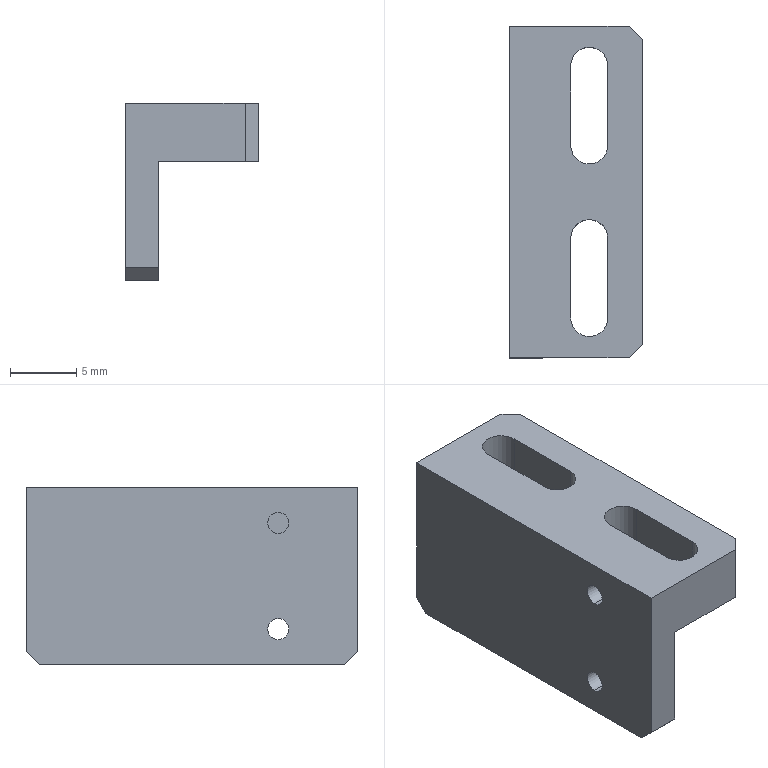Part | SolidWorks | features Chamfer 1, Cut 1, Extrusion 1, HoleWzd 1, ICE 1 | 1 solid | 24 faces | box 10 x 25 x 13.4 mm | volume 1439 mm3 | plane 16 | cylinder 8 | commonest cylinder face diameters 1.6 x4 2.8 x4
STEP:
#1=CARTESIAN_POINT('',(2.5,6.,-9.9));
#2=VERTEX_POINT('',#1);
#3=CARTESIAN_POINT('',(2.5,6.,-11.5));
#4=VERTEX_POINT('',#3);
#5=CARTESIAN_POINT('',(2.5,6.,-10.7));
#6=DIRECTION('',(1.,0.,0.));
#7=DIRECTION('',(0.,0.,1.));
#8=AXIS2_PLACEMENT_3D('',#5,#6,#7);
#9=CIRCLE('',#8,0.8);
#10=EDGE_CURVE('',#2,#4,#9,.T.);
#11=ORIENTED_EDGE('',*,*,#10,.T.);
#12=CARTESIAN_POINT('',(0.,6.,-11.5));
#13=VERTEX_POINT('',#12);
#14=CARTESIAN_POINT('',(0.,6.,-11.5));
#15=DIRECTION('',(-1.,0.,0.));
#16=VECTOR('',#15,1000.);
#17=LINE('',#14,#16);
#18=EDGE_CURVE('',#4,#13,#17,.T.);
#19=ORIENTED_EDGE('',*,*,#18,.T.);
#20=CARTESIAN_POINT('',(0.,6.,-9.9));
#21=VERTEX_POINT('',#20);
#22=CARTESIAN_POINT('',(0.,6.,-10.7));
#23=DIRECTION('',(-1.,0.,0.));
#24=DIRECTION('',(0.,0.,1.));
#25=AXIS2_PLACEMENT_3D('',#22,#23,#24);
#26=CIRCLE('',#25,0.8);
#27=EDGE_CURVE('',#13,#21,#26,.T.);
#28=ORIENTED_EDGE('',*,*,#27,.T.);
#29=CARTESIAN_POINT('',(0.,6.,-9.9));
#30=DIRECTION('',(-1.,0.,0.));
#31=VECTOR('',#30,1000.);
#32=LINE('',#29,#31);
#33=EDGE_CURVE('',#2,#21,#32,.T.);
#34=ORIENTED_EDGE('',*,*,#33,.F.);
#35=EDGE_LOOP('',(#11,#19,#28,#34));
#36=FACE_OUTER_BOUND('',#35,.T.);
#37=CARTESIAN_POINT('',(0.,6.,-10.7));
#38=DIRECTION('',(-1.,0.,0.));
#39=DIRECTION('',(0.,0.,1.));
#40=AXIS2_PLACEMENT_3D('',#37,#38,#39);
#41=CYLINDRICAL_SURFACE('',#40,0.8);
#42=ADVANCED_FACE('',(#36),#41,.F.);
#43=CARTESIAN_POINT('',(4.6,6.,-3.5));
#44=VERTEX_POINT('',#43);
#45=CARTESIAN_POINT('',(4.6,6.,-1.9));
#46=VERTEX_POINT('',#45);
#47=CARTESIAN_POINT('',(4.6,6.,-2.7));
#48=DIRECTION('',(-1.,0.,0.));
#49=DIRECTION('',(0.,0.,1.));
#50=AXIS2_PLACEMENT_3D('',#47,#48,#49);
#51=CIRCLE('',#50,0.8);
#52=EDGE_CURVE('',#44,#46,#51,.T.);
#53=ORIENTED_EDGE('',*,*,#52,.F.);
#54=CARTESIAN_POINT('',(0.,6.,-3.5));
#55=VERTEX_POINT('',#54);
#56=CARTESIAN_POINT('',(0.,6.,-3.5));
#57=DIRECTION('',(-1.,0.,0.));
#58=VECTOR('',#57,1000.);
#59=LINE('',#56,#58);
#60=EDGE_CURVE('',#44,#55,#59,.T.);
#61=ORIENTED_EDGE('',*,*,#60,.T.);
#62=CARTESIAN_POINT('',(0.,6.,-1.9));
#63=VERTEX_POINT('',#62);
#64=CARTESIAN_POINT('',(0.,6.,-2.7));
#65=DIRECTION('',(-1.,0.,0.));
#66=DIRECTION('',(0.,0.,1.));
#67=AXIS2_PLACEMENT_3D('',#64,#65,#66);
#68=CIRCLE('',#67,0.8);
#69=EDGE_CURVE('',#55,#63,#68,.T.);
#70=ORIENTED_EDGE('',*,*,#69,.T.);
#71=CARTESIAN_POINT('',(0.,6.,-1.9));
#72=DIRECTION('',(-1.,0.,0.));
#73=VECTOR('',#72,1000.);
#74=LINE('',#71,#73);
#75=EDGE_CURVE('',#46,#63,#74,.T.);
#76=ORIENTED_EDGE('',*,*,#75,.F.);
#77=EDGE_LOOP('',(#53,#61,#70,#76));
#78=FACE_OUTER_BOUND('',#77,.T.);
#79=CARTESIAN_POINT('',(0.,6.,-2.7));
#80=DIRECTION('',(-1.,0.,0.));
#81=DIRECTION('',(0.,0.,1.));
#82=AXIS2_PLACEMENT_3D('',#79,#80,#81);
#83=CYLINDRICAL_SURFACE('',#82,0.8);
#84=ADVANCED_FACE('',(#78),#83,.F.);
#85=CARTESIAN_POINT('',(0.,6.,-10.7));
#86=DIRECTION('',(-1.,0.,0.));
#87=DIRECTION('',(0.,0.,1.));
#88=AXIS2_PLACEMENT_3D('',#85,#86,#87);
#89=CIRCLE('',#88,0.8);
#90=EDGE_CURVE('',#21,#13,#89,.T.);
#91=ORIENTED_EDGE('',*,*,#90,.F.);
#92=ORIENTED_EDGE('',*,*,#27,.F.);
#93=EDGE_LOOP('',(#91,#92));
#94=FACE_BOUND('',#93,.T.);
#95=CARTESIAN_POINT('',(0.,6.,-2.7));
#96=DIRECTION('',(-1.,0.,0.));
#97=DIRECTION('',(0.,0.,1.));
#98=AXIS2_PLACEMENT_3D('',#95,#96,#97);
#99=CIRCLE('',#98,0.8);
#100=EDGE_CURVE('',#63,#55,#99,.T.);
#101=ORIENTED_EDGE('',*,*,#100,.F.);
#102=ORIENTED_EDGE('',*,*,#69,.F.);
#103=EDGE_LOOP('',(#101,#102));
#104=FACE_BOUND('',#103,.T.);
#105=CARTESIAN_POINT('',(0.,24.,-13.4));
#106=VERTEX_POINT('',#105);
#107=CARTESIAN_POINT('',(0.,1.,-13.4));
#108=VERTEX_POINT('',#107);
#109=CARTESIAN_POINT('',(0.,25.,-13.4));
#110=DIRECTION('',(0.,-1.,0.));
#111=VECTOR('',#110,1000.);
#112=LINE('',#109,#111);
#113=EDGE_CURVE('',#106,#108,#112,.T.);
#114=ORIENTED_EDGE('',*,*,#113,.T.);
#115=CARTESIAN_POINT('',(0.,0.,-12.4));
#116=VERTEX_POINT('',#115);
#117=CARTESIAN_POINT('',(0.,1.,-13.4));
#118=DIRECTION('',(0.,-0.7071,0.7071));
#119=VECTOR('',#118,1000.);
#120=LINE('',#117,#119);
#121=EDGE_CURVE('',#108,#116,#120,.T.);
#122=ORIENTED_EDGE('',*,*,#121,.T.);
#123=CARTESIAN_POINT('',(0.,0.,0.));
#124=VERTEX_POINT('',#123);
#125=CARTESIAN_POINT('',(0.,0.,0.));
#126=DIRECTION('',(0.,0.,1.));
#127=VECTOR('',#126,1000.);
#128=LINE('',#125,#127);
#129=EDGE_CURVE('',#116,#124,#128,.T.);
#130=ORIENTED_EDGE('',*,*,#129,.T.);
#131=CARTESIAN_POINT('',(0.,25.,0.));
#132=VERTEX_POINT('',#131);
#133=CARTESIAN_POINT('',(0.,25.,0.));
#134=DIRECTION('',(0.,-1.,0.));
#135=VECTOR('',#134,1000.);
#136=LINE('',#133,#135);
#137=EDGE_CURVE('',#132,#124,#136,.T.);
#138=ORIENTED_EDGE('',*,*,#137,.F.);
#139=CARTESIAN_POINT('',(0.,25.,-12.4));
#140=VERTEX_POINT('',#139);
#141=CARTESIAN_POINT('',(0.,25.,0.));
#142=DIRECTION('',(0.,0.,1.));
#143=VECTOR('',#142,1000.);
#144=LINE('',#141,#143);
#145=EDGE_CURVE('',#140,#132,#144,.T.);
#146=ORIENTED_EDGE('',*,*,#145,.F.);
#147=CARTESIAN_POINT('',(0.,25.,-12.4));
#148=DIRECTION('',(0.,-0.7071,-0.7071));
#149=VECTOR('',#148,1000.);
#150=LINE('',#147,#149);
#151=EDGE_CURVE('',#140,#106,#150,.T.);
#152=ORIENTED_EDGE('',*,*,#151,.T.);
#153=EDGE_LOOP('',(#114,#122,#130,#138,#146,#152));
#154=FACE_OUTER_BOUND('',#153,.T.);
#155=CARTESIAN_POINT('',(0.,25.,0.));
#156=DIRECTION('',(1.,0.,0.));
#157=DIRECTION('',(0.,0.,-1.));
#158=AXIS2_PLACEMENT_3D('',#155,#156,#157);
#159=PLANE('',#158);
#160=ADVANCED_FACE('',(#94,#104,#154),#159,.F.);
#161=CARTESIAN_POINT('',(7.4,3.,0.));
#162=VERTEX_POINT('',#161);
#163=CARTESIAN_POINT('',(7.4,9.,0.));
#164=VERTEX_POINT('',#163);
#165=CARTESIAN_POINT('',(7.4,3.,0.));
#166=DIRECTION('',(0.,1.,0.));
#167=VECTOR('',#166,1000.);
#168=LINE('',#165,#167);
#169=EDGE_CURVE('',#162,#164,#168,.T.);
#170=ORIENTED_EDGE('',*,*,#169,.F.);
#171=CARTESIAN_POINT('',(4.6,3.,0.));
#172=VERTEX_POINT('',#171);
#173=CARTESIAN_POINT('',(6.,3.,0.));
#174=DIRECTION('',(0.,0.,1.));
#175=DIRECTION('',(-1.,0.,0.));
#176=AXIS2_PLACEMENT_3D('',#173,#174,#175);
#177=CIRCLE('',#176,1.4);
#178=EDGE_CURVE('',#172,#162,#177,.T.);
#179=ORIENTED_EDGE('',*,*,#178,.F.);
#180=CARTESIAN_POINT('',(4.6,9.,0.));
#181=VERTEX_POINT('',#180);
#182=CARTESIAN_POINT('',(4.6,3.,0.));
#183=DIRECTION('',(0.,-1.,0.));
#184=VECTOR('',#183,1000.);
#185=LINE('',#182,#184);
#186=EDGE_CURVE('',#181,#172,#185,.T.);
#187=ORIENTED_EDGE('',*,*,#186,.F.);
#188=CARTESIAN_POINT('',(6.,9.,0.));
#189=DIRECTION('',(0.,0.,1.));
#190=DIRECTION('',(-1.,0.,0.));
#191=AXIS2_PLACEMENT_3D('',#188,#189,#190);
#192=CIRCLE('',#191,1.4);
#193=EDGE_CURVE('',#164,#181,#192,.T.);
#194=ORIENTED_EDGE('',*,*,#193,.F.);
#195=EDGE_LOOP('',(#170,#179,#187,#194));
#196=FACE_BOUND('',#195,.T.);
#197=CARTESIAN_POINT('',(4.6,22.,0.));
#198=VERTEX_POINT('',#197);
#199=CARTESIAN_POINT('',(4.6,16.,0.));
#200=VERTEX_POINT('',#199);
#201=CARTESIAN_POINT('',(4.6,22.,0.));
#202=DIRECTION('',(0.,-1.,0.));
#203=VECTOR('',#202,1000.);
#204=LINE('',#201,#203);
#205=EDGE_CURVE('',#198,#200,#204,.T.);
#206=ORIENTED_EDGE('',*,*,#205,.F.);
#207=CARTESIAN_POINT('',(7.4,22.,0.));
#208=VERTEX_POINT('',#207);
#209=CARTESIAN_POINT('',(6.,22.,0.));
#210=DIRECTION('',(0.,0.,1.));
#211=DIRECTION('',(1.,0.,0.));
#212=AXIS2_PLACEMENT_3D('',#209,#210,#211);
#213=CIRCLE('',#212,1.4);
#214=EDGE_CURVE('',#208,#198,#213,.T.);
#215=ORIENTED_EDGE('',*,*,#214,.F.);
#216=CARTESIAN_POINT('',(7.4,16.,0.));
#217=VERTEX_POINT('',#216);
#218=CARTESIAN_POINT('',(7.4,22.,0.));
#219=DIRECTION('',(0.,1.,0.));
#220=VECTOR('',#219,1000.);
#221=LINE('',#218,#220);
#222=EDGE_CURVE('',#217,#208,#221,.T.);
#223=ORIENTED_EDGE('',*,*,#222,.F.);
#224=CARTESIAN_POINT('',(6.,16.,0.));
#225=DIRECTION('',(0.,0.,1.));
#226=DIRECTION('',(1.,0.,0.));
#227=AXIS2_PLACEMENT_3D('',#224,#225,#226);
#228=CIRCLE('',#227,1.4);
#229=EDGE_CURVE('',#200,#217,#228,.T.);
#230=ORIENTED_EDGE('',*,*,#229,.F.);
#231=EDGE_LOOP('',(#206,#215,#223,#230));
#232=FACE_BOUND('',#231,.T.);
#233=CARTESIAN_POINT('',(9.,0.,0.));
#234=VERTEX_POINT('',#233);
#235=CARTESIAN_POINT('',(0.,0.,0.));
#236=DIRECTION('',(1.,0.,0.));
#237=VECTOR('',#236,1000.);
#238=LINE('',#235,#237);
#239=EDGE_CURVE('',#124,#234,#238,.T.);
#240=ORIENTED_EDGE('',*,*,#239,.T.);
#241=CARTESIAN_POINT('',(10.,1.,0.));
#242=VERTEX_POINT('',#241);
#243=CARTESIAN_POINT('',(10.,1.,0.));
#244=DIRECTION('',(0.7071,0.7071,0.));
#245=VECTOR('',#244,1000.);
#246=LINE('',#243,#245);
#247=EDGE_CURVE('',#234,#242,#246,.T.);
#248=ORIENTED_EDGE('',*,*,#247,.T.);
#249=CARTESIAN_POINT('',(10.,24.,0.));
#250=VERTEX_POINT('',#249);
#251=CARTESIAN_POINT('',(10.,25.,0.));
#252=DIRECTION('',(0.,-1.,0.));
#253=VECTOR('',#252,1000.);
#254=LINE('',#251,#253);
#255=EDGE_CURVE('',#250,#242,#254,.T.);
#256=ORIENTED_EDGE('',*,*,#255,.F.);
#257=CARTESIAN_POINT('',(9.,25.,0.));
#258=VERTEX_POINT('',#257);
#259=CARTESIAN_POINT('',(9.,25.,0.));
#260=DIRECTION('',(-0.7071,0.7071,0.));
#261=VECTOR('',#260,1000.);
#262=LINE('',#259,#261);
#263=EDGE_CURVE('',#250,#258,#262,.T.);
#264=ORIENTED_EDGE('',*,*,#263,.T.);
#265=CARTESIAN_POINT('',(0.,25.,0.));
#266=DIRECTION('',(1.,0.,0.));
#267=VECTOR('',#266,1000.);
#268=LINE('',#265,#267);
#269=EDGE_CURVE('',#132,#258,#268,.T.);
#270=ORIENTED_EDGE('',*,*,#269,.F.);
#271=ORIENTED_EDGE('',*,*,#137,.T.);
#272=EDGE_LOOP('',(#240,#248,#256,#264,#270,#271));
#273=FACE_OUTER_BOUND('',#272,.T.);
#274=CARTESIAN_POINT('',(0.,25.,0.));
#275=DIRECTION('',(0.,0.,-1.));
#276=DIRECTION('',(-1.,0.,0.));
#277=AXIS2_PLACEMENT_3D('',#274,#275,#276);
#278=PLANE('',#277);
#279=ADVANCED_FACE('',(#196,#232,#273),#278,.F.);
#280=ORIENTED_EDGE('',*,*,#255,.T.);
#281=CARTESIAN_POINT('',(10.,1.,-4.4));
#282=VERTEX_POINT('',#281);
#283=CARTESIAN_POINT('',(10.,1.,-4.4));
#284=DIRECTION('',(0.,0.,-1.));
#285=VECTOR('',#284,1000.);
#286=LINE('',#283,#285);
#287=EDGE_CURVE('',#242,#282,#286,.T.);
#288=ORIENTED_EDGE('',*,*,#287,.T.);
#289=CARTESIAN_POINT('',(10.,24.,-4.4));
#290=VERTEX_POINT('',#289);
#291=CARTESIAN_POINT('',(10.,25.,-4.4));
#292=DIRECTION('',(0.,1.,0.));
#293=VECTOR('',#292,1000.);
#294=LINE('',#291,#293);
#295=EDGE_CURVE('',#282,#290,#294,.T.);
#296=ORIENTED_EDGE('',*,*,#295,.T.);
#297=CARTESIAN_POINT('',(10.,24.,0.));
#298=DIRECTION('',(0.,0.,1.));
#299=VECTOR('',#298,1000.);
#300=LINE('',#297,#299);
#301=EDGE_CURVE('',#290,#250,#300,.T.);
#302=ORIENTED_EDGE('',*,*,#301,.T.);
#303=EDGE_LOOP('',(#280,#288,#296,#302));
#304=FACE_OUTER_BOUND('',#303,.T.);
#305=CARTESIAN_POINT('',(10.,25.,0.));
#306=DIRECTION('',(-1.,0.,0.));
#307=DIRECTION('',(0.,0.,1.));
#308=AXIS2_PLACEMENT_3D('',#305,#306,#307);
#309=PLANE('',#308);
#310=ADVANCED_FACE('',(#304),#309,.F.);
#311=CARTESIAN_POINT('',(2.5,1.,-13.4));
#312=VERTEX_POINT('',#311);
#313=CARTESIAN_POINT('',(2.5,24.,-13.4));
#314=VERTEX_POINT('',#313);
#315=CARTESIAN_POINT('',(2.5,25.,-13.4));
#316=DIRECTION('',(0.,1.,0.));
#317=VECTOR('',#316,1000.);
#318=LINE('',#315,#317);
#319=EDGE_CURVE('',#312,#314,#318,.T.);
#320=ORIENTED_EDGE('',*,*,#319,.F.);
#321=CARTESIAN_POINT('',(0.,1.,-13.4));
#322=DIRECTION('',(-1.,0.,0.));
#323=VECTOR('',#322,1000.);
#324=LINE('',#321,#323);
#325=EDGE_CURVE('',#312,#108,#324,.T.);
#326=ORIENTED_EDGE('',*,*,#325,.T.);
#327=ORIENTED_EDGE('',*,*,#113,.F.);
#328=CARTESIAN_POINT('',(0.,24.,-13.4));
#329=DIRECTION('',(1.,0.,0.));
#330=VECTOR('',#329,1000.);
#331=LINE('',#328,#330);
#332=EDGE_CURVE('',#106,#314,#331,.T.);
#333=ORIENTED_EDGE('',*,*,#332,.T.);
#334=EDGE_LOOP('',(#320,#326,#327,#333));
#335=FACE_OUTER_BOUND('',#334,.T.);
#336=CARTESIAN_POINT('',(0.,25.,-13.4));
#337=DIRECTION('',(0.,0.,1.));
#338=DIRECTION('',(1.,0.,0.));
#339=AXIS2_PLACEMENT_3D('',#336,#337,#338);
#340=PLANE('',#339);
#341=ADVANCED_FACE('',(#335),#340,.F.);
#342=CARTESIAN_POINT('',(2.5,25.,-4.4));
#343=VERTEX_POINT('',#342);
#344=CARTESIAN_POINT('',(2.5,25.,-12.4));
#345=VERTEX_POINT('',#344);
#346=CARTESIAN_POINT('',(2.5,25.,-4.4));
#347=DIRECTION('',(0.,0.,-1.));
#348=VECTOR('',#347,1000.);
#349=LINE('',#346,#348);
#350=EDGE_CURVE('',#343,#345,#349,.T.);
#351=ORIENTED_EDGE('',*,*,#350,.T.);
#352=CARTESIAN_POINT('',(0.,25.,-12.4));
#353=DIRECTION('',(-1.,0.,0.));
#354=VECTOR('',#353,1000.);
#355=LINE('',#352,#354);
#356=EDGE_CURVE('',#345,#140,#355,.T.);
#357=ORIENTED_EDGE('',*,*,#356,.T.);
#358=ORIENTED_EDGE('',*,*,#145,.T.);
#359=ORIENTED_EDGE('',*,*,#269,.T.);
#360=CARTESIAN_POINT('',(9.,25.,-4.4));
#361=VERTEX_POINT('',#360);
#362=CARTESIAN_POINT('',(9.,25.,0.));
#363=DIRECTION('',(0.,0.,-1.));
#364=VECTOR('',#363,1000.);
#365=LINE('',#362,#364);
#366=EDGE_CURVE('',#258,#361,#365,.T.);
#367=ORIENTED_EDGE('',*,*,#366,.T.);
#368=CARTESIAN_POINT('',(2.5,25.,-4.4));
#369=DIRECTION('',(1.,0.,0.));
#370=VECTOR('',#369,1000.);
#371=LINE('',#368,#370);
#372=EDGE_CURVE('',#343,#361,#371,.T.);
#373=ORIENTED_EDGE('',*,*,#372,.F.);
#374=EDGE_LOOP('',(#351,#357,#358,#359,#367,#373));
#375=FACE_OUTER_BOUND('',#374,.T.);
#376=CARTESIAN_POINT('',(0.,25.,0.));
#377=DIRECTION('',(0.,-1.,0.));
#378=DIRECTION('',(0.,0.,-1.));
#379=AXIS2_PLACEMENT_3D('',#376,#377,#378);
#380=PLANE('',#379);
#381=ADVANCED_FACE('',(#375),#380,.F.);
#382=ORIENTED_EDGE('',*,*,#129,.F.);
#383=CARTESIAN_POINT('',(2.5,0.,-12.4));
#384=VERTEX_POINT('',#383);
#385=CARTESIAN_POINT('',(2.5,0.,-12.4));
#386=DIRECTION('',(1.,0.,0.));
#387=VECTOR('',#386,1000.);
#388=LINE('',#385,#387);
#389=EDGE_CURVE('',#116,#384,#388,.T.);
#390=ORIENTED_EDGE('',*,*,#389,.T.);
#391=CARTESIAN_POINT('',(2.5,0.,-4.4));
#392=VERTEX_POINT('',#391);
#393=CARTESIAN_POINT('',(2.5,0.,-4.4));
#394=DIRECTION('',(0.,0.,-1.));
#395=VECTOR('',#394,1000.);
#396=LINE('',#393,#395);
#397=EDGE_CURVE('',#392,#384,#396,.T.);
#398=ORIENTED_EDGE('',*,*,#397,.F.);
#399=CARTESIAN_POINT('',(9.,0.,-4.4));
#400=VERTEX_POINT('',#399);
#401=CARTESIAN_POINT('',(2.5,0.,-4.4));
#402=DIRECTION('',(-1.,0.,0.));
#403=VECTOR('',#402,1000.);
#404=LINE('',#401,#403);
#405=EDGE_CURVE('',#400,#392,#404,.T.);
#406=ORIENTED_EDGE('',*,*,#405,.F.);
#407=CARTESIAN_POINT('',(9.,0.,0.));
#408=DIRECTION('',(0.,0.,1.));
#409=VECTOR('',#408,1000.);
#410=LINE('',#407,#409);
#411=EDGE_CURVE('',#400,#234,#410,.T.);
#412=ORIENTED_EDGE('',*,*,#411,.T.);
#413=ORIENTED_EDGE('',*,*,#239,.F.);
#414=EDGE_LOOP('',(#382,#390,#398,#406,#412,#413));
#415=FACE_OUTER_BOUND('',#414,.T.);
#416=CARTESIAN_POINT('',(0.,0.,0.));
#417=DIRECTION('',(0.,-1.,0.));
#418=DIRECTION('',(0.,0.,-1.));
#419=AXIS2_PLACEMENT_3D('',#416,#417,#418);
#420=PLANE('',#419);
#421=ADVANCED_FACE('',(#415),#420,.T.);
#422=CARTESIAN_POINT('',(4.6,22.,-4.4));
#423=VERTEX_POINT('',#422);
#424=CARTESIAN_POINT('',(4.6,22.,-14.));
#425=DIRECTION('',(0.,0.,1.));
#426=VECTOR('',#425,1000.);
#427=LINE('',#424,#426);
#428=EDGE_CURVE('',#423,#198,#427,.T.);
#429=ORIENTED_EDGE('',*,*,#428,.F.);
#430=CARTESIAN_POINT('',(7.4,22.,-4.4));
#431=VERTEX_POINT('',#430);
#432=CARTESIAN_POINT('',(6.,22.,-4.4));
#433=DIRECTION('',(0.,0.,-1.));
#434=DIRECTION('',(1.,0.,0.));
#435=AXIS2_PLACEMENT_3D('',#432,#433,#434);
#436=CIRCLE('',#435,1.4);
#437=EDGE_CURVE('',#423,#431,#436,.T.);
#438=ORIENTED_EDGE('',*,*,#437,.T.);
#439=CARTESIAN_POINT('',(7.4,22.,-14.));
#440=DIRECTION('',(0.,0.,1.));
#441=VECTOR('',#440,1000.);
#442=LINE('',#439,#441);
#443=EDGE_CURVE('',#431,#208,#442,.T.);
#444=ORIENTED_EDGE('',*,*,#443,.T.);
#445=ORIENTED_EDGE('',*,*,#214,.T.);
#446=EDGE_LOOP('',(#429,#438,#444,#445));
#447=FACE_OUTER_BOUND('',#446,.T.);
#448=CARTESIAN_POINT('',(6.,22.,-14.));
#449=DIRECTION('',(0.,0.,1.));
#450=DIRECTION('',(1.,0.,0.));
#451=AXIS2_PLACEMENT_3D('',#448,#449,#450);
#452=CYLINDRICAL_SURFACE('',#451,1.4);
#453=ADVANCED_FACE('',(#447),#452,.F.);
#454=ORIENTED_EDGE('',*,*,#443,.F.);
#455=CARTESIAN_POINT('',(7.4,16.,-4.4));
#456=VERTEX_POINT('',#455);
#457=CARTESIAN_POINT('',(7.4,22.,-4.4));
#458=DIRECTION('',(0.,-1.,0.));
#459=VECTOR('',#458,1000.);
#460=LINE('',#457,#459);
#461=EDGE_CURVE('',#431,#456,#460,.T.);
#462=ORIENTED_EDGE('',*,*,#461,.T.);
#463=CARTESIAN_POINT('',(7.4,16.,-14.));
#464=DIRECTION('',(0.,0.,1.));
#465=VECTOR('',#464,1000.);
#466=LINE('',#463,#465);
#467=EDGE_CURVE('',#456,#217,#466,.T.);
#468=ORIENTED_EDGE('',*,*,#467,.T.);
#469=ORIENTED_EDGE('',*,*,#222,.T.);
#470=EDGE_LOOP('',(#454,#462,#468,#469));
#471=FACE_OUTER_BOUND('',#470,.T.);
#472=CARTESIAN_POINT('',(7.4,22.,-14.));
#473=DIRECTION('',(1.,0.,0.));
#474=DIRECTION('',(0.,0.,-1.));
#475=AXIS2_PLACEMENT_3D('',#472,#473,#474);
#476=PLANE('',#475);
#477=ADVANCED_FACE('',(#471),#476,.F.);
#478=ORIENTED_EDGE('',*,*,#467,.F.);
#479=CARTESIAN_POINT('',(4.6,16.,-4.4));
#480=VERTEX_POINT('',#479);
#481=CARTESIAN_POINT('',(6.,16.,-4.4));
#482=DIRECTION('',(0.,0.,-1.));
#483=DIRECTION('',(1.,0.,0.));
#484=AXIS2_PLACEMENT_3D('',#481,#482,#483);
#485=CIRCLE('',#484,1.4);
#486=EDGE_CURVE('',#456,#480,#485,.T.);
#487=ORIENTED_EDGE('',*,*,#486,.T.);
#488=CARTESIAN_POINT('',(4.6,16.,-14.));
#489=DIRECTION('',(0.,0.,1.));
#490=VECTOR('',#489,1000.);
#491=LINE('',#488,#490);
#492=EDGE_CURVE('',#480,#200,#491,.T.);
#493=ORIENTED_EDGE('',*,*,#492,.T.);
#494=ORIENTED_EDGE('',*,*,#229,.T.);
#495=EDGE_LOOP('',(#478,#487,#493,#494));
#496=FACE_OUTER_BOUND('',#495,.T.);
#497=CARTESIAN_POINT('',(6.,16.,-14.));
#498=DIRECTION('',(0.,0.,1.));
#499=DIRECTION('',(1.,0.,0.));
#500=AXIS2_PLACEMENT_3D('',#497,#498,#499);
#501=CYLINDRICAL_SURFACE('',#500,1.4);
#502=ADVANCED_FACE('',(#496),#501,.F.);
#503=ORIENTED_EDGE('',*,*,#492,.F.);
#504=CARTESIAN_POINT('',(4.6,22.,-4.4));
#505=DIRECTION('',(0.,1.,0.));
#506=VECTOR('',#505,1000.);
#507=LINE('',#504,#506);
#508=EDGE_CURVE('',#480,#423,#507,.T.);
#509=ORIENTED_EDGE('',*,*,#508,.T.);
#510=ORIENTED_EDGE('',*,*,#428,.T.);
#511=ORIENTED_EDGE('',*,*,#205,.T.);
#512=EDGE_LOOP('',(#503,#509,#510,#511));
#513=FACE_OUTER_BOUND('',#512,.T.);
#514=CARTESIAN_POINT('',(4.6,22.,-14.));
#515=DIRECTION('',(-1.,0.,0.));
#516=DIRECTION('',(0.,0.,1.));
#517=AXIS2_PLACEMENT_3D('',#514,#515,#516);
#518=PLANE('',#517);
#519=ADVANCED_FACE('',(#513),#518,.F.);
#520=CARTESIAN_POINT('',(7.4,3.,-4.4));
#521=VERTEX_POINT('',#520);
#522=CARTESIAN_POINT('',(7.4,3.,-14.));
#523=DIRECTION('',(0.,0.,1.));
#524=VECTOR('',#523,1000.);
#525=LINE('',#522,#524);
#526=EDGE_CURVE('',#521,#162,#525,.T.);
#527=ORIENTED_EDGE('',*,*,#526,.F.);
#528=CARTESIAN_POINT('',(4.6,3.,-4.4));
#529=VERTEX_POINT('',#528);
#530=CARTESIAN_POINT('',(6.,3.,-4.4));
#531=DIRECTION('',(0.,0.,-1.));
#532=DIRECTION('',(1.,0.,0.));
#533=AXIS2_PLACEMENT_3D('',#530,#531,#532);
#534=CIRCLE('',#533,1.4);
#535=EDGE_CURVE('',#521,#529,#534,.T.);
#536=ORIENTED_EDGE('',*,*,#535,.T.);
#537=CARTESIAN_POINT('',(4.6,3.,-14.));
#538=DIRECTION('',(0.,0.,1.));
#539=VECTOR('',#538,1000.);
#540=LINE('',#537,#539);
#541=EDGE_CURVE('',#529,#172,#540,.T.);
#542=ORIENTED_EDGE('',*,*,#541,.T.);
#543=ORIENTED_EDGE('',*,*,#178,.T.);
#544=EDGE_LOOP('',(#527,#536,#542,#543));
#545=FACE_OUTER_BOUND('',#544,.T.);
#546=CARTESIAN_POINT('',(6.,3.,-14.));
#547=DIRECTION('',(0.,0.,1.));
#548=DIRECTION('',(1.,0.,0.));
#549=AXIS2_PLACEMENT_3D('',#546,#547,#548);
#550=CYLINDRICAL_SURFACE('',#549,1.4);
#551=ADVANCED_FACE('',(#545),#550,.F.);
#552=CARTESIAN_POINT('',(4.6,6.,-2.7));
#553=DIRECTION('',(-1.,0.,0.));
#554=DIRECTION('',(0.,0.,1.));
#555=AXIS2_PLACEMENT_3D('',#552,#553,#554);
#556=CIRCLE('',#555,0.8);
#557=EDGE_CURVE('',#46,#44,#556,.T.);
#558=ORIENTED_EDGE('',*,*,#557,.T.);
#559=ORIENTED_EDGE('',*,*,#52,.T.);
#560=EDGE_LOOP('',(#558,#559));
#561=FACE_BOUND('',#560,.T.);
#562=ORIENTED_EDGE('',*,*,#541,.F.);
#563=CARTESIAN_POINT('',(4.6,9.,-4.4));
#564=VERTEX_POINT('',#563);
#565=CARTESIAN_POINT('',(4.6,3.,-4.4));
#566=DIRECTION('',(0.,1.,0.));
#567=VECTOR('',#566,1000.);
#568=LINE('',#565,#567);
#569=EDGE_CURVE('',#529,#564,#568,.T.);
#570=ORIENTED_EDGE('',*,*,#569,.T.);
#571=CARTESIAN_POINT('',(4.6,9.,-14.));
#572=DIRECTION('',(0.,0.,1.));
#573=VECTOR('',#572,1000.);
#574=LINE('',#571,#573);
#575=EDGE_CURVE('',#564,#181,#574,.T.);
#576=ORIENTED_EDGE('',*,*,#575,.T.);
#577=ORIENTED_EDGE('',*,*,#186,.T.);
#578=EDGE_LOOP('',(#562,#570,#576,#577));
#579=FACE_OUTER_BOUND('',#578,.T.);
#580=CARTESIAN_POINT('',(4.6,3.,-14.));
#581=DIRECTION('',(-1.,0.,0.));
#582=DIRECTION('',(0.,0.,1.));
#583=AXIS2_PLACEMENT_3D('',#580,#581,#582);
#584=PLANE('',#583);
#585=ADVANCED_FACE('',(#561,#579),#584,.F.);
#586=ORIENTED_EDGE('',*,*,#575,.F.);
#587=CARTESIAN_POINT('',(7.4,9.,-4.4));
#588=VERTEX_POINT('',#587);
#589=CARTESIAN_POINT('',(6.,9.,-4.4));
#590=DIRECTION('',(0.,0.,-1.));
#591=DIRECTION('',(1.,0.,0.));
#592=AXIS2_PLACEMENT_3D('',#589,#590,#591);
#593=CIRCLE('',#592,1.4);
#594=EDGE_CURVE('',#564,#588,#593,.T.);
#595=ORIENTED_EDGE('',*,*,#594,.T.);
#596=CARTESIAN_POINT('',(7.4,9.,-14.));
#597=DIRECTION('',(0.,0.,1.));
#598=VECTOR('',#597,1000.);
#599=LINE('',#596,#598);
#600=EDGE_CURVE('',#588,#164,#599,.T.);
#601=ORIENTED_EDGE('',*,*,#600,.T.);
#602=ORIENTED_EDGE('',*,*,#193,.T.);
#603=EDGE_LOOP('',(#586,#595,#601,#602));
#604=FACE_OUTER_BOUND('',#603,.T.);
#605=CARTESIAN_POINT('',(6.,9.,-14.));
#606=DIRECTION('',(0.,0.,1.));
#607=DIRECTION('',(1.,0.,0.));
#608=AXIS2_PLACEMENT_3D('',#605,#606,#607);
#609=CYLINDRICAL_SURFACE('',#608,1.4);
#610=ADVANCED_FACE('',(#604),#609,.F.);
#611=ORIENTED_EDGE('',*,*,#600,.F.);
#612=CARTESIAN_POINT('',(7.4,3.,-4.4));
#613=DIRECTION('',(0.,-1.,0.));
#614=VECTOR('',#613,1000.);
#615=LINE('',#612,#614);
#616=EDGE_CURVE('',#588,#521,#615,.T.);
#617=ORIENTED_EDGE('',*,*,#616,.T.);
#618=ORIENTED_EDGE('',*,*,#526,.T.);
#619=ORIENTED_EDGE('',*,*,#169,.T.);
#620=EDGE_LOOP('',(#611,#617,#618,#619));
#621=FACE_OUTER_BOUND('',#620,.T.);
#622=CARTESIAN_POINT('',(7.4,3.,-14.));
#623=DIRECTION('',(1.,0.,0.));
#624=DIRECTION('',(0.,0.,-1.));
#625=AXIS2_PLACEMENT_3D('',#622,#623,#624);
#626=PLANE('',#625);
#627=ADVANCED_FACE('',(#621),#626,.F.);
#628=ORIENTED_EDGE('',*,*,#60,.F.);
#629=ORIENTED_EDGE('',*,*,#557,.F.);
#630=ORIENTED_EDGE('',*,*,#75,.T.);
#631=ORIENTED_EDGE('',*,*,#100,.T.);
#632=EDGE_LOOP('',(#628,#629,#630,#631));
#633=FACE_OUTER_BOUND('',#632,.T.);
#634=CARTESIAN_POINT('',(0.,6.,-2.7));
#635=DIRECTION('',(-1.,0.,0.));
#636=DIRECTION('',(0.,0.,1.));
#637=AXIS2_PLACEMENT_3D('',#634,#635,#636);
#638=CYLINDRICAL_SURFACE('',#637,0.8);
#639=ADVANCED_FACE('',(#633),#638,.F.);
#640=ORIENTED_EDGE('',*,*,#18,.F.);
#641=CARTESIAN_POINT('',(2.5,6.,-10.7));
#642=DIRECTION('',(1.,0.,0.));
#643=DIRECTION('',(0.,0.,1.));
#644=AXIS2_PLACEMENT_3D('',#641,#642,#643);
#645=CIRCLE('',#644,0.8);
#646=EDGE_CURVE('',#4,#2,#645,.T.);
#647=ORIENTED_EDGE('',*,*,#646,.T.);
#648=ORIENTED_EDGE('',*,*,#33,.T.);
#649=ORIENTED_EDGE('',*,*,#90,.T.);
#650=EDGE_LOOP('',(#640,#647,#648,#649));
#651=FACE_OUTER_BOUND('',#650,.T.);
#652=CARTESIAN_POINT('',(0.,6.,-10.7));
#653=DIRECTION('',(-1.,0.,0.));
#654=DIRECTION('',(0.,0.,1.));
#655=AXIS2_PLACEMENT_3D('',#652,#653,#654);
#656=CYLINDRICAL_SURFACE('',#655,0.8);
#657=ADVANCED_FACE('',(#651),#656,.F.);
#658=ORIENTED_EDGE('',*,*,#508,.F.);
#659=ORIENTED_EDGE('',*,*,#486,.F.);
#660=ORIENTED_EDGE('',*,*,#461,.F.);
#661=ORIENTED_EDGE('',*,*,#437,.F.);
#662=EDGE_LOOP('',(#658,#659,#660,#661));
#663=FACE_BOUND('',#662,.T.);
#664=ORIENTED_EDGE('',*,*,#616,.F.);
#665=ORIENTED_EDGE('',*,*,#594,.F.);
#666=ORIENTED_EDGE('',*,*,#569,.F.);
#667=ORIENTED_EDGE('',*,*,#535,.F.);
#668=EDGE_LOOP('',(#664,#665,#666,#667));
#669=FACE_BOUND('',#668,.T.);
#670=ORIENTED_EDGE('',*,*,#295,.F.);
#671=CARTESIAN_POINT('',(10.,1.,-4.4));
#672=DIRECTION('',(-0.7071,-0.7071,0.));
#673=VECTOR('',#672,1000.);
#674=LINE('',#671,#673);
#675=EDGE_CURVE('',#282,#400,#674,.T.);
#676=ORIENTED_EDGE('',*,*,#675,.T.);
#677=ORIENTED_EDGE('',*,*,#405,.T.);
#678=CARTESIAN_POINT('',(2.5,25.,-4.4));
#679=DIRECTION('',(0.,1.,0.));
#680=VECTOR('',#679,1000.);
#681=LINE('',#678,#680);
#682=EDGE_CURVE('',#392,#343,#681,.T.);
#683=ORIENTED_EDGE('',*,*,#682,.T.);
#684=ORIENTED_EDGE('',*,*,#372,.T.);
#685=CARTESIAN_POINT('',(9.,25.,-4.4));
#686=DIRECTION('',(0.7071,-0.7071,0.));
#687=VECTOR('',#686,1000.);
#688=LINE('',#685,#687);
#689=EDGE_CURVE('',#361,#290,#688,.T.);
#690=ORIENTED_EDGE('',*,*,#689,.T.);
#691=EDGE_LOOP('',(#670,#676,#677,#683,#684,#690));
#692=FACE_OUTER_BOUND('',#691,.T.);
#693=CARTESIAN_POINT('',(0.,0.,-4.4));
#694=DIRECTION('',(0.,0.,1.));
#695=DIRECTION('',(1.,0.,0.));
#696=AXIS2_PLACEMENT_3D('',#693,#694,#695);
#697=PLANE('',#696);
#698=ADVANCED_FACE('',(#663,#669,#692),#697,.F.);
#699=ORIENTED_EDGE('',*,*,#397,.T.);
#700=CARTESIAN_POINT('',(2.5,1.,-13.4));
#701=DIRECTION('',(0.,0.7071,-0.7071));
#702=VECTOR('',#701,1000.);
#703=LINE('',#700,#702);
#704=EDGE_CURVE('',#384,#312,#703,.T.);
#705=ORIENTED_EDGE('',*,*,#704,.T.);
#706=ORIENTED_EDGE('',*,*,#319,.T.);
#707=CARTESIAN_POINT('',(2.5,25.,-12.4));
#708=DIRECTION('',(0.,0.7071,0.7071));
#709=VECTOR('',#708,1000.);
#710=LINE('',#707,#709);
#711=EDGE_CURVE('',#314,#345,#710,.T.);
#712=ORIENTED_EDGE('',*,*,#711,.T.);
#713=ORIENTED_EDGE('',*,*,#350,.F.);
#714=ORIENTED_EDGE('',*,*,#682,.F.);
#715=EDGE_LOOP('',(#699,#705,#706,#712,#713,#714));
#716=FACE_OUTER_BOUND('',#715,.T.);
#717=ORIENTED_EDGE('',*,*,#10,.F.);
#718=ORIENTED_EDGE('',*,*,#646,.F.);
#719=EDGE_LOOP('',(#717,#718));
#720=FACE_BOUND('',#719,.T.);
#721=CARTESIAN_POINT('',(2.5,25.,-4.4));
#722=DIRECTION('',(-1.,0.,0.));
#723=DIRECTION('',(0.,0.,1.));
#724=AXIS2_PLACEMENT_3D('',#721,#722,#723);
#725=PLANE('',#724);
#726=ADVANCED_FACE('',(#716,#720),#725,.F.);
#727=ORIENTED_EDGE('',*,*,#704,.F.);
#728=ORIENTED_EDGE('',*,*,#389,.F.);
#729=ORIENTED_EDGE('',*,*,#121,.F.);
#730=ORIENTED_EDGE('',*,*,#325,.F.);
#731=EDGE_LOOP('',(#727,#728,#729,#730));
#732=FACE_OUTER_BOUND('',#731,.T.);
#733=CARTESIAN_POINT('',(0.,1.,-13.4));
#734=DIRECTION('',(0.,-0.7071,-0.7071));
#735=DIRECTION('',(1.,0.,0.));
#736=AXIS2_PLACEMENT_3D('',#733,#734,#735);
#737=PLANE('',#736);
#738=ADVANCED_FACE('',(#732),#737,.T.);
#739=ORIENTED_EDGE('',*,*,#711,.F.);
#740=ORIENTED_EDGE('',*,*,#332,.F.);
#741=ORIENTED_EDGE('',*,*,#151,.F.);
#742=ORIENTED_EDGE('',*,*,#356,.F.);
#743=EDGE_LOOP('',(#739,#740,#741,#742));
#744=FACE_OUTER_BOUND('',#743,.T.);
#745=CARTESIAN_POINT('',(0.,25.,-12.4));
#746=DIRECTION('',(0.,-0.7071,0.7071));
#747=DIRECTION('',(-1.,0.,0.));
#748=AXIS2_PLACEMENT_3D('',#745,#746,#747);
#749=PLANE('',#748);
#750=ADVANCED_FACE('',(#744),#749,.F.);
#751=ORIENTED_EDGE('',*,*,#247,.F.);
#752=ORIENTED_EDGE('',*,*,#411,.F.);
#753=ORIENTED_EDGE('',*,*,#675,.F.);
#754=ORIENTED_EDGE('',*,*,#287,.F.);
#755=EDGE_LOOP('',(#751,#752,#753,#754));
#756=FACE_OUTER_BOUND('',#755,.T.);
#757=CARTESIAN_POINT('',(10.,1.,0.));
#758=DIRECTION('',(0.7071,-0.7071,0.));
#759=DIRECTION('',(0.,0.,1.));
#760=AXIS2_PLACEMENT_3D('',#757,#758,#759);
#761=PLANE('',#760);
#762=ADVANCED_FACE('',(#756),#761,.T.);
#763=ORIENTED_EDGE('',*,*,#263,.F.);
#764=ORIENTED_EDGE('',*,*,#301,.F.);
#765=ORIENTED_EDGE('',*,*,#689,.F.);
#766=ORIENTED_EDGE('',*,*,#366,.F.);
#767=EDGE_LOOP('',(#763,#764,#765,#766));
#768=FACE_OUTER_BOUND('',#767,.T.);
#769=CARTESIAN_POINT('',(9.,25.,0.));
#770=DIRECTION('',(-0.7071,-0.7071,0.));
#771=DIRECTION('',(0.,0.,-1.));
#772=AXIS2_PLACEMENT_3D('',#769,#770,#771);
#773=PLANE('',#772);
#774=ADVANCED_FACE('',(#768),#773,.F.);
#775=CLOSED_SHELL('',(#42,#84,#160,#279,#310,#341,#381,#421,#453,#477,#502,#519,#551,#585,#610,#627,#639,#657,#698,#726,#738,#750,#762,#774));
#776=MANIFOLD_SOLID_BREP('',#775);
#777=CARTESIAN_POINT('',(0.,0.,0.));
#778=DIRECTION('',(0.,0.,1.));
#779=DIRECTION('',(1.,0.,0.));
#780=AXIS2_PLACEMENT_3D('',#777,#778,#779);
#781=(LENGTH_UNIT()NAMED_UNIT(*)SI_UNIT(.MILLI.,.METRE.));
#782=UNCERTAINTY_MEASURE_WITH_UNIT(LENGTH_MEASURE(0.00001),#781,'','');
#783=(NAMED_UNIT(*)PLANE_ANGLE_UNIT()SI_UNIT($,.RADIAN.));
#784=(NAMED_UNIT(*)SI_UNIT($,.STERADIAN.)SOLID_ANGLE_UNIT());
#785=(GEOMETRIC_REPRESENTATION_CONTEXT(3)GLOBAL_UNCERTAINTY_ASSIGNED_CONTEXT((#782))GLOBAL_UNIT_ASSIGNED_CONTEXT((#781,#783,#784))REPRESENTATION_CONTEXT('',''));
#786=ADVANCED_BREP_SHAPE_REPRESENTATION('',(#776,#780),#785);